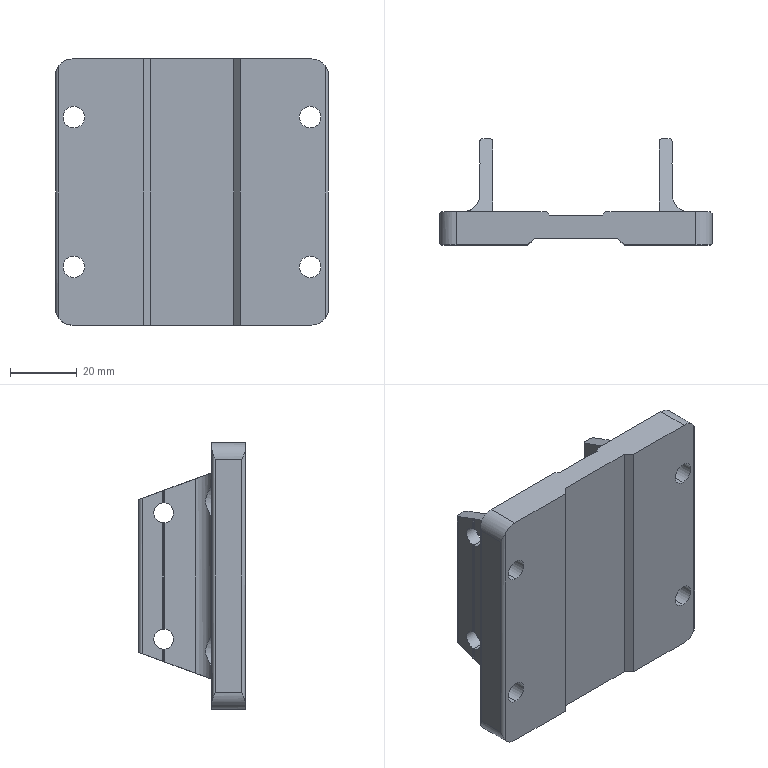Part | STEP file | Copy of 50N support base^K50A-1H20-S(formula driven)-L300-motor left- | 1 solid | 107 faces | box 82 x 32 x 80 mm | volume 67767 mm3 | cylinder 55 | plane 52 | commonest cylinder face diameters 0.2 x21 2 x8 6 x8 6.5 x8 10 x6 11 x4